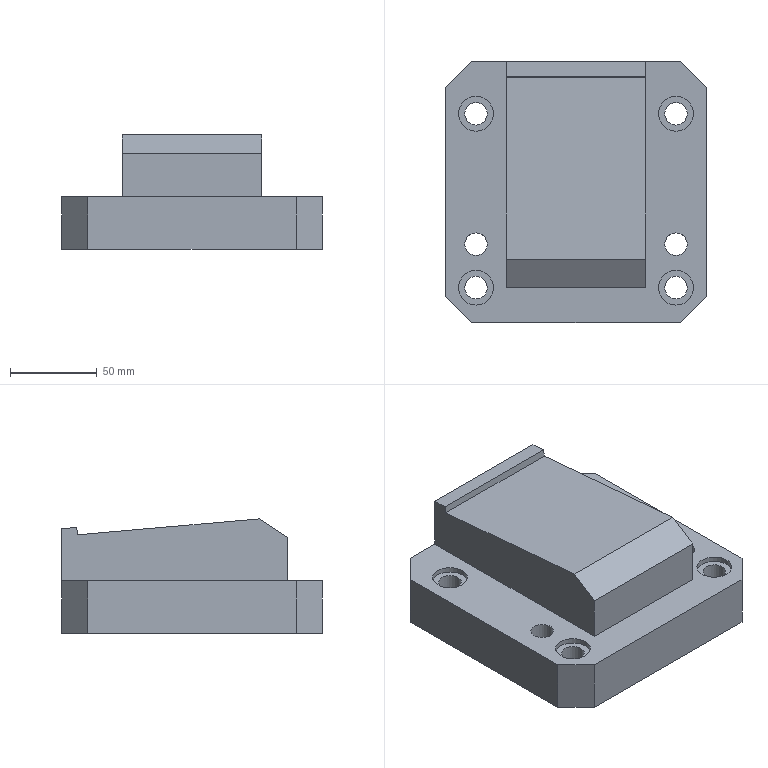Part | NX | features solid 2 | 1 solid | 40 faces | box 150 x 150 x 65.685 mm | volume 939891 mm3 | plane 30 | cylinder 10 | commonest cylinder face diameters 13 x6 20 x4
STEP:
#1=CARTESIAN_POINT('',(197.5,-243.5,-135.));
#2=VERTEX_POINT('',#1);
#3=CARTESIAN_POINT('',(197.5,-250.,-135.));
#4=DIRECTION('',(0.,0.,1.));
#5=DIRECTION('',(0.,1.,0.));
#6=AXIS2_PLACEMENT_3D('',#3,#4,#5);
#7=CIRCLE('',#6,6.5);
#8=EDGE_CURVE('',#2,#2,#7,.T.);
#9=ORIENTED_EDGE('',*,*,#8,.F.);
#10=EDGE_LOOP('',(#9));
#11=FACE_BOUND('',#10,.T.);
#12=CARTESIAN_POINT('',(82.5,-243.5,-135.));
#13=VERTEX_POINT('',#12);
#14=CARTESIAN_POINT('',(82.5,-250.,-135.));
#15=DIRECTION('',(0.,0.,1.));
#16=DIRECTION('',(0.,1.,0.));
#17=AXIS2_PLACEMENT_3D('',#14,#15,#16);
#18=CIRCLE('',#17,6.5);
#19=EDGE_CURVE('',#13,#13,#18,.T.);
#20=ORIENTED_EDGE('',*,*,#19,.F.);
#21=EDGE_LOOP('',(#20));
#22=FACE_BOUND('',#21,.T.);
#23=CARTESIAN_POINT('',(197.5,-265.,-135.));
#24=VERTEX_POINT('',#23);
#25=CARTESIAN_POINT('',(197.5,-275.,-135.));
#26=DIRECTION('',(0.,0.,1.));
#27=DIRECTION('',(0.,1.,0.));
#28=AXIS2_PLACEMENT_3D('',#25,#26,#27);
#29=CIRCLE('',#28,10.);
#30=EDGE_CURVE('',#24,#24,#29,.T.);
#31=ORIENTED_EDGE('',*,*,#30,.F.);
#32=EDGE_LOOP('',(#31));
#33=FACE_BOUND('',#32,.T.);
#34=CARTESIAN_POINT('',(197.5,-165.,-135.));
#35=VERTEX_POINT('',#34);
#36=CARTESIAN_POINT('',(197.5,-175.,-135.));
#37=DIRECTION('',(0.,0.,1.));
#38=DIRECTION('',(0.,1.,0.));
#39=AXIS2_PLACEMENT_3D('',#36,#37,#38);
#40=CIRCLE('',#39,10.);
#41=EDGE_CURVE('',#35,#35,#40,.T.);
#42=ORIENTED_EDGE('',*,*,#41,.F.);
#43=EDGE_LOOP('',(#42));
#44=FACE_BOUND('',#43,.T.);
#45=CARTESIAN_POINT('',(82.5,-165.,-135.));
#46=VERTEX_POINT('',#45);
#47=CARTESIAN_POINT('',(82.5,-175.,-135.));
#48=DIRECTION('',(0.,0.,1.));
#49=DIRECTION('',(0.,1.,0.));
#50=AXIS2_PLACEMENT_3D('',#47,#48,#49);
#51=CIRCLE('',#50,10.);
#52=EDGE_CURVE('',#46,#46,#51,.T.);
#53=ORIENTED_EDGE('',*,*,#52,.F.);
#54=EDGE_LOOP('',(#53));
#55=FACE_BOUND('',#54,.T.);
#56=CARTESIAN_POINT('',(82.5,-265.,-135.));
#57=VERTEX_POINT('',#56);
#58=CARTESIAN_POINT('',(82.5,-275.,-135.));
#59=DIRECTION('',(0.,0.,1.));
#60=DIRECTION('',(0.,1.,0.));
#61=AXIS2_PLACEMENT_3D('',#58,#59,#60);
#62=CIRCLE('',#61,10.);
#63=EDGE_CURVE('',#57,#57,#62,.T.);
#64=ORIENTED_EDGE('',*,*,#63,.F.);
#65=EDGE_LOOP('',(#64));
#66=FACE_BOUND('',#65,.T.);
#67=CARTESIAN_POINT('',(180.,-275.,-135.));
#68=VERTEX_POINT('',#67);
#69=CARTESIAN_POINT('',(100.,-275.,-135.));
#70=VERTEX_POINT('',#69);
#71=CARTESIAN_POINT('',(180.,-275.,-135.));
#72=DIRECTION('',(-1.,0.,0.));
#73=VECTOR('',#72,1000.);
#74=LINE('',#71,#73);
#75=EDGE_CURVE('',#68,#70,#74,.T.);
#76=ORIENTED_EDGE('',*,*,#75,.T.);
#77=CARTESIAN_POINT('',(100.,-145.,-135.));
#78=VERTEX_POINT('',#77);
#79=CARTESIAN_POINT('',(100.,-295.,-135.));
#80=DIRECTION('',(0.,1.,0.));
#81=VECTOR('',#80,1000.);
#82=LINE('',#79,#81);
#83=EDGE_CURVE('',#70,#78,#82,.T.);
#84=ORIENTED_EDGE('',*,*,#83,.T.);
#85=CARTESIAN_POINT('',(80.,-145.,-135.));
#86=VERTEX_POINT('',#85);
#87=CARTESIAN_POINT('',(215.,-145.,-135.));
#88=DIRECTION('',(-1.,0.,0.));
#89=VECTOR('',#88,1000.);
#90=LINE('',#87,#89);
#91=EDGE_CURVE('',#78,#86,#90,.T.);
#92=ORIENTED_EDGE('',*,*,#91,.T.);
#93=CARTESIAN_POINT('',(65.,-160.,-135.));
#94=VERTEX_POINT('',#93);
#95=CARTESIAN_POINT('',(72.5,-152.5,-135.));
#96=DIRECTION('',(0.7071,0.7071,0.));
#97=VECTOR('',#96,1000.);
#98=LINE('',#95,#97);
#99=EDGE_CURVE('',#86,#94,#98,.F.);
#100=ORIENTED_EDGE('',*,*,#99,.T.);
#101=CARTESIAN_POINT('',(65.,-280.,-135.));
#102=VERTEX_POINT('',#101);
#103=CARTESIAN_POINT('',(65.,-295.,-135.));
#104=DIRECTION('',(0.,1.,0.));
#105=VECTOR('',#104,1000.);
#106=LINE('',#103,#105);
#107=EDGE_CURVE('',#102,#94,#106,.T.);
#108=ORIENTED_EDGE('',*,*,#107,.F.);
#109=CARTESIAN_POINT('',(80.,-295.,-135.));
#110=VERTEX_POINT('',#109);
#111=CARTESIAN_POINT('',(147.5,-362.5,-135.));
#112=DIRECTION('',(0.7071,-0.7071,0.));
#113=VECTOR('',#112,1000.);
#114=LINE('',#111,#113);
#115=EDGE_CURVE('',#102,#110,#114,.T.);
#116=ORIENTED_EDGE('',*,*,#115,.T.);
#117=CARTESIAN_POINT('',(200.,-295.,-135.));
#118=VERTEX_POINT('',#117);
#119=CARTESIAN_POINT('',(215.,-295.,-135.));
#120=DIRECTION('',(-1.,0.,0.));
#121=VECTOR('',#120,1000.);
#122=LINE('',#119,#121);
#123=EDGE_CURVE('',#118,#110,#122,.T.);
#124=ORIENTED_EDGE('',*,*,#123,.F.);
#125=CARTESIAN_POINT('',(215.,-280.,-135.));
#126=VERTEX_POINT('',#125);
#127=CARTESIAN_POINT('',(207.5,-287.5,-135.));
#128=DIRECTION('',(-0.7071,-0.7071,0.));
#129=VECTOR('',#128,1000.);
#130=LINE('',#127,#129);
#131=EDGE_CURVE('',#118,#126,#130,.F.);
#132=ORIENTED_EDGE('',*,*,#131,.T.);
#133=CARTESIAN_POINT('',(215.,-160.,-135.));
#134=VERTEX_POINT('',#133);
#135=CARTESIAN_POINT('',(215.,-295.,-135.));
#136=DIRECTION('',(0.,1.,0.));
#137=VECTOR('',#136,1000.);
#138=LINE('',#135,#137);
#139=EDGE_CURVE('',#126,#134,#138,.T.);
#140=ORIENTED_EDGE('',*,*,#139,.T.);
#141=CARTESIAN_POINT('',(200.,-145.,-135.));
#142=VERTEX_POINT('',#141);
#143=CARTESIAN_POINT('',(282.5,-227.5,-135.));
#144=DIRECTION('',(-0.7071,0.7071,0.));
#145=VECTOR('',#144,1000.);
#146=LINE('',#143,#145);
#147=EDGE_CURVE('',#134,#142,#146,.T.);
#148=ORIENTED_EDGE('',*,*,#147,.T.);
#149=CARTESIAN_POINT('',(180.,-145.,-135.));
#150=VERTEX_POINT('',#149);
#151=CARTESIAN_POINT('',(215.,-145.,-135.));
#152=DIRECTION('',(-1.,0.,0.));
#153=VECTOR('',#152,1000.);
#154=LINE('',#151,#153);
#155=EDGE_CURVE('',#142,#150,#154,.T.);
#156=ORIENTED_EDGE('',*,*,#155,.T.);
#157=CARTESIAN_POINT('',(180.,-295.,-135.));
#158=DIRECTION('',(0.,1.,0.));
#159=VECTOR('',#158,1000.);
#160=LINE('',#157,#159);
#161=EDGE_CURVE('',#68,#150,#160,.T.);
#162=ORIENTED_EDGE('',*,*,#161,.F.);
#163=EDGE_LOOP('',(#76,#84,#92,#100,#108,#116,#124,#132,#140,#148,#156,#162));
#164=FACE_BOUND('',#163,.T.);
#165=CARTESIAN_POINT('',(215.,-295.,-135.));
#166=DIRECTION('',(0.,0.,1.));
#167=DIRECTION('',(0.,1.,0.));
#168=AXIS2_PLACEMENT_3D('',#165,#166,#167);
#169=PLANE('',#168);
#170=ADVANCED_FACE('',(#11,#22,#33,#44,#55,#66,#164),#169,.T.);
#171=CARTESIAN_POINT('',(200.,-145.,-165.));
#172=VERTEX_POINT('',#171);
#173=CARTESIAN_POINT('',(80.,-145.,-165.));
#174=VERTEX_POINT('',#173);
#175=CARTESIAN_POINT('',(215.,-145.,-165.));
#176=DIRECTION('',(-1.,0.,0.));
#177=VECTOR('',#176,1000.);
#178=LINE('',#175,#177);
#179=EDGE_CURVE('',#172,#174,#178,.T.);
#180=ORIENTED_EDGE('',*,*,#179,.T.);
#181=CARTESIAN_POINT('',(80.,-145.,-135.));
#182=DIRECTION('',(0.,0.,1.));
#183=VECTOR('',#182,1000.);
#184=LINE('',#181,#183);
#185=EDGE_CURVE('',#174,#86,#184,.T.);
#186=ORIENTED_EDGE('',*,*,#185,.T.);
#187=ORIENTED_EDGE('',*,*,#91,.F.);
#188=CARTESIAN_POINT('',(100.,-145.,-105.));
#189=VERTEX_POINT('',#188);
#190=CARTESIAN_POINT('',(100.,-145.,-135.));
#191=DIRECTION('',(0.,0.,1.));
#192=VECTOR('',#191,1000.);
#193=LINE('',#190,#192);
#194=EDGE_CURVE('',#78,#189,#193,.T.);
#195=ORIENTED_EDGE('',*,*,#194,.T.);
#196=CARTESIAN_POINT('',(180.,-145.,-105.));
#197=VERTEX_POINT('',#196);
#198=CARTESIAN_POINT('',(180.,-145.,-105.));
#199=DIRECTION('',(-1.,0.,0.));
#200=VECTOR('',#199,1000.);
#201=LINE('',#198,#200);
#202=EDGE_CURVE('',#197,#189,#201,.T.);
#203=ORIENTED_EDGE('',*,*,#202,.F.);
#204=CARTESIAN_POINT('',(180.,-145.,-135.));
#205=DIRECTION('',(0.,0.,1.));
#206=VECTOR('',#205,1000.);
#207=LINE('',#204,#206);
#208=EDGE_CURVE('',#150,#197,#207,.T.);
#209=ORIENTED_EDGE('',*,*,#208,.F.);
#210=ORIENTED_EDGE('',*,*,#155,.F.);
#211=CARTESIAN_POINT('',(200.,-145.,-165.));
#212=DIRECTION('',(0.,0.,-1.));
#213=VECTOR('',#212,1000.);
#214=LINE('',#211,#213);
#215=EDGE_CURVE('',#142,#172,#214,.T.);
#216=ORIENTED_EDGE('',*,*,#215,.T.);
#217=EDGE_LOOP('',(#180,#186,#187,#195,#203,#209,#210,#216));
#218=FACE_BOUND('',#217,.T.);
#219=CARTESIAN_POINT('',(215.,-145.,-135.));
#220=DIRECTION('',(0.,1.,0.));
#221=DIRECTION('',(0.,0.,-1.));
#222=AXIS2_PLACEMENT_3D('',#219,#220,#221);
#223=PLANE('',#222);
#224=ADVANCED_FACE('',(#218),#223,.T.);
#225=CARTESIAN_POINT('',(197.5,-181.5,-165.));
#226=VERTEX_POINT('',#225);
#227=CARTESIAN_POINT('',(197.5,-175.,-165.));
#228=DIRECTION('',(0.,0.,-1.));
#229=DIRECTION('',(0.,-1.,0.));
#230=AXIS2_PLACEMENT_3D('',#227,#228,#229);
#231=CIRCLE('',#230,6.5);
#232=EDGE_CURVE('',#226,#226,#231,.T.);
#233=ORIENTED_EDGE('',*,*,#232,.F.);
#234=EDGE_LOOP('',(#233));
#235=FACE_BOUND('',#234,.T.);
#236=CARTESIAN_POINT('',(82.5,-256.5,-165.));
#237=VERTEX_POINT('',#236);
#238=CARTESIAN_POINT('',(82.5,-250.,-165.));
#239=DIRECTION('',(0.,0.,-1.));
#240=DIRECTION('',(0.,-1.,0.));
#241=AXIS2_PLACEMENT_3D('',#238,#239,#240);
#242=CIRCLE('',#241,6.5);
#243=EDGE_CURVE('',#237,#237,#242,.T.);
#244=ORIENTED_EDGE('',*,*,#243,.F.);
#245=EDGE_LOOP('',(#244));
#246=FACE_BOUND('',#245,.T.);
#247=CARTESIAN_POINT('',(82.5,-281.5,-165.));
#248=VERTEX_POINT('',#247);
#249=CARTESIAN_POINT('',(82.5,-275.,-165.));
#250=DIRECTION('',(0.,0.,-1.));
#251=DIRECTION('',(0.,-1.,0.));
#252=AXIS2_PLACEMENT_3D('',#249,#250,#251);
#253=CIRCLE('',#252,6.5);
#254=EDGE_CURVE('',#248,#248,#253,.T.);
#255=ORIENTED_EDGE('',*,*,#254,.F.);
#256=EDGE_LOOP('',(#255));
#257=FACE_BOUND('',#256,.T.);
#258=CARTESIAN_POINT('',(82.5,-181.5,-165.));
#259=VERTEX_POINT('',#258);
#260=CARTESIAN_POINT('',(82.5,-175.,-165.));
#261=DIRECTION('',(0.,0.,-1.));
#262=DIRECTION('',(0.,-1.,0.));
#263=AXIS2_PLACEMENT_3D('',#260,#261,#262);
#264=CIRCLE('',#263,6.5);
#265=EDGE_CURVE('',#259,#259,#264,.T.);
#266=ORIENTED_EDGE('',*,*,#265,.F.);
#267=EDGE_LOOP('',(#266));
#268=FACE_BOUND('',#267,.T.);
#269=CARTESIAN_POINT('',(197.5,-256.5,-165.));
#270=VERTEX_POINT('',#269);
#271=CARTESIAN_POINT('',(197.5,-250.,-165.));
#272=DIRECTION('',(0.,0.,-1.));
#273=DIRECTION('',(0.,-1.,0.));
#274=AXIS2_PLACEMENT_3D('',#271,#272,#273);
#275=CIRCLE('',#274,6.5);
#276=EDGE_CURVE('',#270,#270,#275,.T.);
#277=ORIENTED_EDGE('',*,*,#276,.F.);
#278=EDGE_LOOP('',(#277));
#279=FACE_BOUND('',#278,.T.);
#280=CARTESIAN_POINT('',(197.5,-281.5,-165.));
#281=VERTEX_POINT('',#280);
#282=CARTESIAN_POINT('',(197.5,-275.,-165.));
#283=DIRECTION('',(0.,0.,-1.));
#284=DIRECTION('',(0.,-1.,0.));
#285=AXIS2_PLACEMENT_3D('',#282,#283,#284);
#286=CIRCLE('',#285,6.5);
#287=EDGE_CURVE('',#281,#281,#286,.T.);
#288=ORIENTED_EDGE('',*,*,#287,.F.);
#289=EDGE_LOOP('',(#288));
#290=FACE_BOUND('',#289,.T.);
#291=CARTESIAN_POINT('',(130.,-250.,-165.));
#292=VERTEX_POINT('',#291);
#293=CARTESIAN_POINT('',(125.,-245.,-165.));
#294=VERTEX_POINT('',#293);
#295=CARTESIAN_POINT('',(125.,-245.,-165.));
#296=DIRECTION('',(0.7071,-0.7071,0.));
#297=VECTOR('',#296,1000.);
#298=LINE('',#295,#297);
#299=EDGE_CURVE('',#292,#294,#298,.F.);
#300=ORIENTED_EDGE('',*,*,#299,.F.);
#301=CARTESIAN_POINT('',(150.,-250.,-165.));
#302=VERTEX_POINT('',#301);
#303=CARTESIAN_POINT('',(125.,-250.,-165.));
#304=DIRECTION('',(-1.,0.,0.));
#305=VECTOR('',#304,1000.);
#306=LINE('',#303,#305);
#307=EDGE_CURVE('',#292,#302,#306,.F.);
#308=ORIENTED_EDGE('',*,*,#307,.T.);
#309=CARTESIAN_POINT('',(155.,-245.,-165.));
#310=VERTEX_POINT('',#309);
#311=CARTESIAN_POINT('',(150.,-250.,-165.));
#312=DIRECTION('',(-0.7071,-0.7071,0.));
#313=VECTOR('',#312,1000.);
#314=LINE('',#311,#313);
#315=EDGE_CURVE('',#310,#302,#314,.T.);
#316=ORIENTED_EDGE('',*,*,#315,.F.);
#317=CARTESIAN_POINT('',(155.,-195.,-165.));
#318=VERTEX_POINT('',#317);
#319=CARTESIAN_POINT('',(155.,-160.,-165.));
#320=DIRECTION('',(0.,-1.,0.));
#321=VECTOR('',#320,1000.);
#322=LINE('',#319,#321);
#323=EDGE_CURVE('',#318,#310,#322,.T.);
#324=ORIENTED_EDGE('',*,*,#323,.F.);
#325=CARTESIAN_POINT('',(150.,-190.,-165.));
#326=VERTEX_POINT('',#325);
#327=CARTESIAN_POINT('',(155.,-195.,-165.));
#328=DIRECTION('',(-0.7071,0.7071,0.));
#329=VECTOR('',#328,1000.);
#330=LINE('',#327,#329);
#331=EDGE_CURVE('',#326,#318,#330,.F.);
#332=ORIENTED_EDGE('',*,*,#331,.F.);
#333=CARTESIAN_POINT('',(130.,-190.,-165.));
#334=VERTEX_POINT('',#333);
#335=CARTESIAN_POINT('',(125.,-190.,-165.));
#336=DIRECTION('',(1.,0.,0.));
#337=VECTOR('',#336,1000.);
#338=LINE('',#335,#337);
#339=EDGE_CURVE('',#334,#326,#338,.T.);
#340=ORIENTED_EDGE('',*,*,#339,.F.);
#341=CARTESIAN_POINT('',(125.,-195.,-165.));
#342=VERTEX_POINT('',#341);
#343=CARTESIAN_POINT('',(130.,-190.,-165.));
#344=DIRECTION('',(0.7071,0.7071,0.));
#345=VECTOR('',#344,1000.);
#346=LINE('',#343,#345);
#347=EDGE_CURVE('',#342,#334,#346,.T.);
#348=ORIENTED_EDGE('',*,*,#347,.F.);
#349=CARTESIAN_POINT('',(125.,-160.,-165.));
#350=DIRECTION('',(0.,-1.,0.));
#351=VECTOR('',#350,1000.);
#352=LINE('',#349,#351);
#353=EDGE_CURVE('',#342,#294,#352,.T.);
#354=ORIENTED_EDGE('',*,*,#353,.T.);
#355=EDGE_LOOP('',(#300,#308,#316,#324,#332,#340,#348,#354));
#356=FACE_BOUND('',#355,.T.);
#357=CARTESIAN_POINT('',(200.,-295.,-165.));
#358=VERTEX_POINT('',#357);
#359=CARTESIAN_POINT('',(80.,-295.,-165.));
#360=VERTEX_POINT('',#359);
#361=CARTESIAN_POINT('',(215.,-295.,-165.));
#362=DIRECTION('',(-1.,0.,0.));
#363=VECTOR('',#362,1000.);
#364=LINE('',#361,#363);
#365=EDGE_CURVE('',#358,#360,#364,.T.);
#366=ORIENTED_EDGE('',*,*,#365,.T.);
#367=CARTESIAN_POINT('',(65.,-280.,-165.));
#368=VERTEX_POINT('',#367);
#369=CARTESIAN_POINT('',(72.5,-287.5,-165.));
#370=DIRECTION('',(-0.7071,0.7071,0.));
#371=VECTOR('',#370,1000.);
#372=LINE('',#369,#371);
#373=EDGE_CURVE('',#360,#368,#372,.T.);
#374=ORIENTED_EDGE('',*,*,#373,.T.);
#375=CARTESIAN_POINT('',(65.,-160.,-165.));
#376=VERTEX_POINT('',#375);
#377=CARTESIAN_POINT('',(65.,-145.,-165.));
#378=DIRECTION('',(0.,-1.,0.));
#379=VECTOR('',#378,1000.);
#380=LINE('',#377,#379);
#381=EDGE_CURVE('',#376,#368,#380,.T.);
#382=ORIENTED_EDGE('',*,*,#381,.F.);
#383=CARTESIAN_POINT('',(147.5,-77.5,-165.));
#384=DIRECTION('',(-0.7071,-0.7071,0.));
#385=VECTOR('',#384,1000.);
#386=LINE('',#383,#385);
#387=EDGE_CURVE('',#376,#174,#386,.F.);
#388=ORIENTED_EDGE('',*,*,#387,.T.);
#389=ORIENTED_EDGE('',*,*,#179,.F.);
#390=CARTESIAN_POINT('',(215.,-160.,-165.));
#391=VERTEX_POINT('',#390);
#392=CARTESIAN_POINT('',(207.5,-152.5,-165.));
#393=DIRECTION('',(0.7071,-0.7071,0.));
#394=VECTOR('',#393,1000.);
#395=LINE('',#392,#394);
#396=EDGE_CURVE('',#172,#391,#395,.T.);
#397=ORIENTED_EDGE('',*,*,#396,.T.);
#398=CARTESIAN_POINT('',(215.,-280.,-165.));
#399=VERTEX_POINT('',#398);
#400=CARTESIAN_POINT('',(215.,-145.,-165.));
#401=DIRECTION('',(0.,-1.,0.));
#402=VECTOR('',#401,1000.);
#403=LINE('',#400,#402);
#404=EDGE_CURVE('',#391,#399,#403,.T.);
#405=ORIENTED_EDGE('',*,*,#404,.T.);
#406=CARTESIAN_POINT('',(282.5,-212.5,-165.));
#407=DIRECTION('',(0.7071,0.7071,0.));
#408=VECTOR('',#407,1000.);
#409=LINE('',#406,#408);
#410=EDGE_CURVE('',#399,#358,#409,.F.);
#411=ORIENTED_EDGE('',*,*,#410,.T.);
#412=EDGE_LOOP('',(#366,#374,#382,#388,#389,#397,#405,#411));
#413=FACE_BOUND('',#412,.T.);
#414=CARTESIAN_POINT('',(215.,-145.,-165.));
#415=DIRECTION('',(0.,0.,-1.));
#416=DIRECTION('',(0.,-1.,0.));
#417=AXIS2_PLACEMENT_3D('',#414,#415,#416);
#418=PLANE('',#417);
#419=ADVANCED_FACE('',(#235,#246,#257,#268,#279,#290,#356,#413),#418,.T.);
#420=ORIENTED_EDGE('',*,*,#123,.T.);
#421=CARTESIAN_POINT('',(80.,-295.,-165.));
#422=DIRECTION('',(0.,0.,-1.));
#423=VECTOR('',#422,1000.);
#424=LINE('',#421,#423);
#425=EDGE_CURVE('',#110,#360,#424,.T.);
#426=ORIENTED_EDGE('',*,*,#425,.T.);
#427=ORIENTED_EDGE('',*,*,#365,.F.);
#428=CARTESIAN_POINT('',(200.,-295.,-135.));
#429=DIRECTION('',(0.,0.,1.));
#430=VECTOR('',#429,1000.);
#431=LINE('',#428,#430);
#432=EDGE_CURVE('',#358,#118,#431,.T.);
#433=ORIENTED_EDGE('',*,*,#432,.T.);
#434=EDGE_LOOP('',(#420,#426,#427,#433));
#435=FACE_BOUND('',#434,.T.);
#436=CARTESIAN_POINT('',(215.,-295.,-135.));
#437=DIRECTION('',(0.,1.,0.));
#438=DIRECTION('',(0.,0.,-1.));
#439=AXIS2_PLACEMENT_3D('',#436,#437,#438);
#440=PLANE('',#439);
#441=ADVANCED_FACE('',(#435),#440,.F.);
#442=ORIENTED_EDGE('',*,*,#404,.F.);
#443=CARTESIAN_POINT('',(215.,-160.,-135.));
#444=DIRECTION('',(0.,0.,1.));
#445=VECTOR('',#444,1000.);
#446=LINE('',#443,#445);
#447=EDGE_CURVE('',#391,#134,#446,.T.);
#448=ORIENTED_EDGE('',*,*,#447,.T.);
#449=ORIENTED_EDGE('',*,*,#139,.F.);
#450=CARTESIAN_POINT('',(215.,-280.,-135.));
#451=DIRECTION('',(0.,0.,-1.));
#452=VECTOR('',#451,1000.);
#453=LINE('',#450,#452);
#454=EDGE_CURVE('',#126,#399,#453,.T.);
#455=ORIENTED_EDGE('',*,*,#454,.T.);
#456=EDGE_LOOP('',(#442,#448,#449,#455));
#457=FACE_BOUND('',#456,.T.);
#458=CARTESIAN_POINT('',(215.,-295.,-135.));
#459=DIRECTION('',(-1.,0.,0.));
#460=DIRECTION('',(0.,0.,1.));
#461=AXIS2_PLACEMENT_3D('',#458,#459,#460);
#462=PLANE('',#461);
#463=ADVANCED_FACE('',(#457),#462,.F.);
#464=ORIENTED_EDGE('',*,*,#381,.T.);
#465=CARTESIAN_POINT('',(65.,-280.,-135.));
#466=DIRECTION('',(0.,0.,1.));
#467=VECTOR('',#466,1000.);
#468=LINE('',#465,#467);
#469=EDGE_CURVE('',#368,#102,#468,.T.);
#470=ORIENTED_EDGE('',*,*,#469,.T.);
#471=ORIENTED_EDGE('',*,*,#107,.T.);
#472=CARTESIAN_POINT('',(65.,-160.,-135.));
#473=DIRECTION('',(0.,0.,-1.));
#474=VECTOR('',#473,1000.);
#475=LINE('',#472,#474);
#476=EDGE_CURVE('',#94,#376,#475,.T.);
#477=ORIENTED_EDGE('',*,*,#476,.T.);
#478=EDGE_LOOP('',(#464,#470,#471,#477));
#479=FACE_BOUND('',#478,.T.);
#480=CARTESIAN_POINT('',(65.,-295.,-135.));
#481=DIRECTION('',(-1.,0.,0.));
#482=DIRECTION('',(0.,0.,1.));
#483=AXIS2_PLACEMENT_3D('',#480,#481,#482);
#484=PLANE('',#483);
#485=ADVANCED_FACE('',(#479),#484,.T.);
#486=ORIENTED_EDGE('',*,*,#115,.F.);
#487=ORIENTED_EDGE('',*,*,#469,.F.);
#488=ORIENTED_EDGE('',*,*,#373,.F.);
#489=ORIENTED_EDGE('',*,*,#425,.F.);
#490=EDGE_LOOP('',(#486,#487,#488,#489));
#491=FACE_BOUND('',#490,.T.);
#492=CARTESIAN_POINT('',(80.,-295.,-135.));
#493=DIRECTION('',(-0.7071,-0.7071,0.));
#494=DIRECTION('',(0.7071,-0.7071,0.));
#495=AXIS2_PLACEMENT_3D('',#492,#493,#494);
#496=PLANE('',#495);
#497=ADVANCED_FACE('',(#491),#496,.T.);
#498=ORIENTED_EDGE('',*,*,#99,.F.);
#499=ORIENTED_EDGE('',*,*,#185,.F.);
#500=ORIENTED_EDGE('',*,*,#387,.F.);
#501=ORIENTED_EDGE('',*,*,#476,.F.);
#502=EDGE_LOOP('',(#498,#499,#500,#501));
#503=FACE_BOUND('',#502,.T.);
#504=CARTESIAN_POINT('',(65.,-160.,-135.));
#505=DIRECTION('',(0.7071,-0.7071,0.));
#506=DIRECTION('',(0.7071,0.7071,0.));
#507=AXIS2_PLACEMENT_3D('',#504,#505,#506);
#508=PLANE('',#507);
#509=ADVANCED_FACE('',(#503),#508,.F.);
#510=ORIENTED_EDGE('',*,*,#147,.F.);
#511=ORIENTED_EDGE('',*,*,#447,.F.);
#512=ORIENTED_EDGE('',*,*,#396,.F.);
#513=ORIENTED_EDGE('',*,*,#215,.F.);
#514=EDGE_LOOP('',(#510,#511,#512,#513));
#515=FACE_BOUND('',#514,.T.);
#516=CARTESIAN_POINT('',(200.,-145.,-135.));
#517=DIRECTION('',(0.7071,0.7071,0.));
#518=DIRECTION('',(-0.7071,0.7071,0.));
#519=AXIS2_PLACEMENT_3D('',#516,#517,#518);
#520=PLANE('',#519);
#521=ADVANCED_FACE('',(#515),#520,.T.);
#522=ORIENTED_EDGE('',*,*,#131,.F.);
#523=ORIENTED_EDGE('',*,*,#432,.F.);
#524=ORIENTED_EDGE('',*,*,#410,.F.);
#525=ORIENTED_EDGE('',*,*,#454,.F.);
#526=EDGE_LOOP('',(#522,#523,#524,#525));
#527=FACE_BOUND('',#526,.T.);
#528=CARTESIAN_POINT('',(215.,-280.,-135.));
#529=DIRECTION('',(-0.7071,0.7071,0.));
#530=DIRECTION('',(-0.7071,-0.7071,0.));
#531=AXIS2_PLACEMENT_3D('',#528,#529,#530);
#532=PLANE('',#531);
#533=ADVANCED_FACE('',(#527),#532,.F.);
#534=ORIENTED_EDGE('',*,*,#353,.F.);
#535=CARTESIAN_POINT('',(125.,-195.,-155.));
#536=VERTEX_POINT('',#535);
#537=CARTESIAN_POINT('',(125.,-195.,-165.));
#538=DIRECTION('',(0.,0.,1.));
#539=VECTOR('',#538,1000.);
#540=LINE('',#537,#539);
#541=EDGE_CURVE('',#536,#342,#540,.F.);
#542=ORIENTED_EDGE('',*,*,#541,.F.);
#543=CARTESIAN_POINT('',(125.,-245.,-155.));
#544=VERTEX_POINT('',#543);
#545=CARTESIAN_POINT('',(125.,-160.,-155.));
#546=DIRECTION('',(0.,1.,0.));
#547=VECTOR('',#546,1000.);
#548=LINE('',#545,#547);
#549=EDGE_CURVE('',#536,#544,#548,.F.);
#550=ORIENTED_EDGE('',*,*,#549,.T.);
#551=CARTESIAN_POINT('',(125.,-245.,-165.));
#552=DIRECTION('',(0.,0.,-1.));
#553=VECTOR('',#552,1000.);
#554=LINE('',#551,#553);
#555=EDGE_CURVE('',#294,#544,#554,.F.);
#556=ORIENTED_EDGE('',*,*,#555,.F.);
#557=EDGE_LOOP('',(#534,#542,#550,#556));
#558=FACE_BOUND('',#557,.T.);
#559=CARTESIAN_POINT('',(125.,-160.,-165.));
#560=DIRECTION('',(-1.,0.,0.));
#561=DIRECTION('',(0.,-1.,0.));
#562=AXIS2_PLACEMENT_3D('',#559,#560,#561);
#563=PLANE('',#562);
#564=ADVANCED_FACE('',(#558),#563,.F.);
#565=ORIENTED_EDGE('',*,*,#339,.T.);
#566=CARTESIAN_POINT('',(150.,-190.,-155.));
#567=VERTEX_POINT('',#566);
#568=CARTESIAN_POINT('',(150.,-190.,-165.));
#569=DIRECTION('',(0.,0.,-1.));
#570=VECTOR('',#569,1000.);
#571=LINE('',#568,#570);
#572=EDGE_CURVE('',#567,#326,#571,.T.);
#573=ORIENTED_EDGE('',*,*,#572,.F.);
#574=CARTESIAN_POINT('',(130.,-190.,-155.));
#575=VERTEX_POINT('',#574);
#576=CARTESIAN_POINT('',(125.,-190.,-155.));
#577=DIRECTION('',(1.,0.,0.));
#578=VECTOR('',#577,1000.);
#579=LINE('',#576,#578);
#580=EDGE_CURVE('',#575,#567,#579,.T.);
#581=ORIENTED_EDGE('',*,*,#580,.F.);
#582=CARTESIAN_POINT('',(130.,-190.,-165.));
#583=DIRECTION('',(0.,0.,1.));
#584=VECTOR('',#583,1000.);
#585=LINE('',#582,#584);
#586=EDGE_CURVE('',#334,#575,#585,.T.);
#587=ORIENTED_EDGE('',*,*,#586,.F.);
#588=EDGE_LOOP('',(#565,#573,#581,#587));
#589=FACE_BOUND('',#588,.T.);
#590=CARTESIAN_POINT('',(125.,-190.,-165.));
#591=DIRECTION('',(0.,-1.,0.));
#592=DIRECTION('',(1.,0.,0.));
#593=AXIS2_PLACEMENT_3D('',#590,#591,#592);
#594=PLANE('',#593);
#595=ADVANCED_FACE('',(#589),#594,.T.);
#596=CARTESIAN_POINT('',(155.,-195.,-155.));
#597=VERTEX_POINT('',#596);
#598=CARTESIAN_POINT('',(155.,-245.,-155.));
#599=VERTEX_POINT('',#598);
#600=CARTESIAN_POINT('',(155.,-160.,-155.));
#601=DIRECTION('',(0.,1.,0.));
#602=VECTOR('',#601,1000.);
#603=LINE('',#600,#602);
#604=EDGE_CURVE('',#597,#599,#603,.F.);
#605=ORIENTED_EDGE('',*,*,#604,.F.);
#606=CARTESIAN_POINT('',(155.,-195.,-165.));
#607=DIRECTION('',(0.,0.,1.));
#608=VECTOR('',#607,1000.);
#609=LINE('',#606,#608);
#610=EDGE_CURVE('',#318,#597,#609,.T.);
#611=ORIENTED_EDGE('',*,*,#610,.F.);
#612=ORIENTED_EDGE('',*,*,#323,.T.);
#613=CARTESIAN_POINT('',(155.,-245.,-165.));
#614=DIRECTION('',(0.,0.,-1.));
#615=VECTOR('',#614,1000.);
#616=LINE('',#613,#615);
#617=EDGE_CURVE('',#599,#310,#616,.T.);
#618=ORIENTED_EDGE('',*,*,#617,.F.);
#619=EDGE_LOOP('',(#605,#611,#612,#618));
#620=FACE_BOUND('',#619,.T.);
#621=CARTESIAN_POINT('',(155.,-160.,-165.));
#622=DIRECTION('',(-1.,0.,0.));
#623=DIRECTION('',(0.,-1.,0.));
#624=AXIS2_PLACEMENT_3D('',#621,#622,#623);
#625=PLANE('',#624);
#626=ADVANCED_FACE('',(#620),#625,.T.);
#627=CARTESIAN_POINT('',(130.,-250.,-155.));
#628=VERTEX_POINT('',#627);
#629=CARTESIAN_POINT('',(150.,-250.,-155.));
#630=VERTEX_POINT('',#629);
#631=CARTESIAN_POINT('',(125.,-250.,-155.));
#632=DIRECTION('',(-1.,0.,0.));
#633=VECTOR('',#632,1000.);
#634=LINE('',#631,#633);
#635=EDGE_CURVE('',#628,#630,#634,.F.);
#636=ORIENTED_EDGE('',*,*,#635,.T.);
#637=CARTESIAN_POINT('',(150.,-250.,-165.));
#638=DIRECTION('',(0.,0.,-1.));
#639=VECTOR('',#638,1000.);
#640=LINE('',#637,#639);
#641=EDGE_CURVE('',#302,#630,#640,.F.);
#642=ORIENTED_EDGE('',*,*,#641,.F.);
#643=ORIENTED_EDGE('',*,*,#307,.F.);
#644=CARTESIAN_POINT('',(130.,-250.,-165.));
#645=DIRECTION('',(0.,0.,1.));
#646=VECTOR('',#645,1000.);
#647=LINE('',#644,#646);
#648=EDGE_CURVE('',#628,#292,#647,.F.);
#649=ORIENTED_EDGE('',*,*,#648,.F.);
#650=EDGE_LOOP('',(#636,#642,#643,#649));
#651=FACE_BOUND('',#650,.T.);
#652=CARTESIAN_POINT('',(125.,-250.,-165.));
#653=DIRECTION('',(0.,-1.,0.));
#654=DIRECTION('',(1.,0.,0.));
#655=AXIS2_PLACEMENT_3D('',#652,#653,#654);
#656=PLANE('',#655);
#657=ADVANCED_FACE('',(#651),#656,.F.);
#658=ORIENTED_EDGE('',*,*,#549,.F.);
#659=CARTESIAN_POINT('',(142.5,-177.5,-155.));
#660=DIRECTION('',(-0.7071,-0.7071,0.));
#661=VECTOR('',#660,1000.);
#662=LINE('',#659,#661);
#663=EDGE_CURVE('',#575,#536,#662,.T.);
#664=ORIENTED_EDGE('',*,*,#663,.F.);
#665=ORIENTED_EDGE('',*,*,#580,.T.);
#666=CARTESIAN_POINT('',(122.5,-162.5,-155.));
#667=DIRECTION('',(0.7071,-0.7071,0.));
#668=VECTOR('',#667,1000.);
#669=LINE('',#666,#668);
#670=EDGE_CURVE('',#597,#567,#669,.F.);
#671=ORIENTED_EDGE('',*,*,#670,.F.);
#672=ORIENTED_EDGE('',*,*,#604,.T.);
#673=CARTESIAN_POINT('',(182.5,-217.5,-155.));
#674=DIRECTION('',(0.7071,0.7071,0.));
#675=VECTOR('',#674,1000.);
#676=LINE('',#673,#675);
#677=EDGE_CURVE('',#630,#599,#676,.T.);
#678=ORIENTED_EDGE('',*,*,#677,.F.);
#679=ORIENTED_EDGE('',*,*,#635,.F.);
#680=CARTESIAN_POINT('',(82.5,-202.5,-155.));
#681=DIRECTION('',(-0.7071,0.7071,0.));
#682=VECTOR('',#681,1000.);
#683=LINE('',#680,#682);
#684=EDGE_CURVE('',#544,#628,#683,.F.);
#685=ORIENTED_EDGE('',*,*,#684,.F.);
#686=EDGE_LOOP('',(#658,#664,#665,#671,#672,#678,#679,#685));
#687=FACE_BOUND('',#686,.T.);
#688=CARTESIAN_POINT('',(125.,-160.,-155.));
#689=DIRECTION('',(0.,0.,1.));
#690=DIRECTION('',(0.,1.,0.));
#691=AXIS2_PLACEMENT_3D('',#688,#689,#690);
#692=PLANE('',#691);
#693=ADVANCED_FACE('',(#687),#692,.F.);
#694=ORIENTED_EDGE('',*,*,#299,.T.);
#695=ORIENTED_EDGE('',*,*,#555,.T.);
#696=ORIENTED_EDGE('',*,*,#684,.T.);
#697=ORIENTED_EDGE('',*,*,#648,.T.);
#698=EDGE_LOOP('',(#694,#695,#696,#697));
#699=FACE_BOUND('',#698,.T.);
#700=CARTESIAN_POINT('',(125.,-245.,-165.));
#701=DIRECTION('',(0.7071,0.7071,0.));
#702=DIRECTION('',(-0.7071,0.7071,0.));
#703=AXIS2_PLACEMENT_3D('',#700,#701,#702);
#704=PLANE('',#703);
#705=ADVANCED_FACE('',(#699),#704,.T.);
#706=ORIENTED_EDGE('',*,*,#315,.T.);
#707=ORIENTED_EDGE('',*,*,#641,.T.);
#708=ORIENTED_EDGE('',*,*,#677,.T.);
#709=ORIENTED_EDGE('',*,*,#617,.T.);
#710=EDGE_LOOP('',(#706,#707,#708,#709));
#711=FACE_BOUND('',#710,.T.);
#712=CARTESIAN_POINT('',(150.,-250.,-165.));
#713=DIRECTION('',(0.7071,-0.7071,0.));
#714=DIRECTION('',(0.7071,0.7071,0.));
#715=AXIS2_PLACEMENT_3D('',#712,#713,#714);
#716=PLANE('',#715);
#717=ADVANCED_FACE('',(#711),#716,.F.);
#718=ORIENTED_EDGE('',*,*,#347,.T.);
#719=ORIENTED_EDGE('',*,*,#586,.T.);
#720=ORIENTED_EDGE('',*,*,#663,.T.);
#721=ORIENTED_EDGE('',*,*,#541,.T.);
#722=EDGE_LOOP('',(#718,#719,#720,#721));
#723=FACE_BOUND('',#722,.T.);
#724=CARTESIAN_POINT('',(130.,-190.,-165.));
#725=DIRECTION('',(-0.7071,0.7071,0.));
#726=DIRECTION('',(-0.7071,-0.7071,0.));
#727=AXIS2_PLACEMENT_3D('',#724,#725,#726);
#728=PLANE('',#727);
#729=ADVANCED_FACE('',(#723),#728,.F.);
#730=ORIENTED_EDGE('',*,*,#331,.T.);
#731=ORIENTED_EDGE('',*,*,#610,.T.);
#732=ORIENTED_EDGE('',*,*,#670,.T.);
#733=ORIENTED_EDGE('',*,*,#572,.T.);
#734=EDGE_LOOP('',(#730,#731,#732,#733));
#735=FACE_BOUND('',#734,.T.);
#736=CARTESIAN_POINT('',(155.,-195.,-165.));
#737=DIRECTION('',(-0.7071,-0.7071,0.));
#738=DIRECTION('',(0.7071,-0.7071,0.));
#739=AXIS2_PLACEMENT_3D('',#736,#737,#738);
#740=PLANE('',#739);
#741=ADVANCED_FACE('',(#735),#740,.T.);
#742=CARTESIAN_POINT('',(197.5,-281.5,-138.));
#743=VERTEX_POINT('',#742);
#744=CARTESIAN_POINT('',(197.5,-275.,-138.));
#745=DIRECTION('',(0.,0.,-1.));
#746=DIRECTION('',(0.,-1.,0.));
#747=AXIS2_PLACEMENT_3D('',#744,#745,#746);
#748=CIRCLE('',#747,6.5);
#749=EDGE_CURVE('',#743,#743,#748,.F.);
#750=ORIENTED_EDGE('',*,*,#749,.T.);
#751=EDGE_LOOP('',(#750));
#752=FACE_BOUND('',#751,.T.);
#753=ORIENTED_EDGE('',*,*,#287,.T.);
#754=EDGE_LOOP('',(#753));
#755=FACE_BOUND('',#754,.T.);
#756=CARTESIAN_POINT('',(197.5,-275.,-24.35));
#757=DIRECTION('',(0.,0.,-1.));
#758=DIRECTION('',(0.,-1.,0.));
#759=AXIS2_PLACEMENT_3D('',#756,#757,#758);
#760=CYLINDRICAL_SURFACE('',#759,6.5);
#761=ADVANCED_FACE('',(#752,#755),#760,.F.);
#762=ORIENTED_EDGE('',*,*,#8,.T.);
#763=EDGE_LOOP('',(#762));
#764=FACE_BOUND('',#763,.T.);
#765=ORIENTED_EDGE('',*,*,#276,.T.);
#766=EDGE_LOOP('',(#765));
#767=FACE_BOUND('',#766,.T.);
#768=CARTESIAN_POINT('',(197.5,-250.,-24.35));
#769=DIRECTION('',(0.,0.,-1.));
#770=DIRECTION('',(0.,-1.,0.));
#771=AXIS2_PLACEMENT_3D('',#768,#769,#770);
#772=CYLINDRICAL_SURFACE('',#771,6.5);
#773=ADVANCED_FACE('',(#764,#767),#772,.F.);
#774=CARTESIAN_POINT('',(82.5,-181.5,-138.));
#775=VERTEX_POINT('',#774);
#776=CARTESIAN_POINT('',(82.5,-175.,-138.));
#777=DIRECTION('',(0.,0.,-1.));
#778=DIRECTION('',(0.,-1.,0.));
#779=AXIS2_PLACEMENT_3D('',#776,#777,#778);
#780=CIRCLE('',#779,6.5);
#781=EDGE_CURVE('',#775,#775,#780,.F.);
#782=ORIENTED_EDGE('',*,*,#781,.T.);
#783=EDGE_LOOP('',(#782));
#784=FACE_BOUND('',#783,.T.);
#785=ORIENTED_EDGE('',*,*,#265,.T.);
#786=EDGE_LOOP('',(#785));
#787=FACE_BOUND('',#786,.T.);
#788=CARTESIAN_POINT('',(82.5,-175.,-24.35));
#789=DIRECTION('',(0.,0.,-1.));
#790=DIRECTION('',(0.,-1.,0.));
#791=AXIS2_PLACEMENT_3D('',#788,#789,#790);
#792=CYLINDRICAL_SURFACE('',#791,6.5);
#793=ADVANCED_FACE('',(#784,#787),#792,.F.);
#794=CARTESIAN_POINT('',(82.5,-281.5,-138.));
#795=VERTEX_POINT('',#794);
#796=CARTESIAN_POINT('',(82.5,-275.,-138.));
#797=DIRECTION('',(0.,0.,-1.));
#798=DIRECTION('',(0.,-1.,0.));
#799=AXIS2_PLACEMENT_3D('',#796,#797,#798);
#800=CIRCLE('',#799,6.5);
#801=EDGE_CURVE('',#795,#795,#800,.F.);
#802=ORIENTED_EDGE('',*,*,#801,.T.);
#803=EDGE_LOOP('',(#802));
#804=FACE_BOUND('',#803,.T.);
#805=ORIENTED_EDGE('',*,*,#254,.T.);
#806=EDGE_LOOP('',(#805));
#807=FACE_BOUND('',#806,.T.);
#808=CARTESIAN_POINT('',(82.5,-275.,-24.35));
#809=DIRECTION('',(0.,0.,-1.));
#810=DIRECTION('',(0.,-1.,0.));
#811=AXIS2_PLACEMENT_3D('',#808,#809,#810);
#812=CYLINDRICAL_SURFACE('',#811,6.5);
#813=ADVANCED_FACE('',(#804,#807),#812,.F.);
#814=ORIENTED_EDGE('',*,*,#19,.T.);
#815=EDGE_LOOP('',(#814));
#816=FACE_BOUND('',#815,.T.);
#817=ORIENTED_EDGE('',*,*,#243,.T.);
#818=EDGE_LOOP('',(#817));
#819=FACE_BOUND('',#818,.T.);
#820=CARTESIAN_POINT('',(82.5,-250.,-24.35));
#821=DIRECTION('',(0.,0.,-1.));
#822=DIRECTION('',(0.,-1.,0.));
#823=AXIS2_PLACEMENT_3D('',#820,#821,#822);
#824=CYLINDRICAL_SURFACE('',#823,6.5);
#825=ADVANCED_FACE('',(#816,#819),#824,.F.);
#826=CARTESIAN_POINT('',(197.5,-181.5,-138.));
#827=VERTEX_POINT('',#826);
#828=CARTESIAN_POINT('',(197.5,-175.,-138.));
#829=DIRECTION('',(0.,0.,-1.));
#830=DIRECTION('',(0.,-1.,0.));
#831=AXIS2_PLACEMENT_3D('',#828,#829,#830);
#832=CIRCLE('',#831,6.5);
#833=EDGE_CURVE('',#827,#827,#832,.F.);
#834=ORIENTED_EDGE('',*,*,#833,.T.);
#835=EDGE_LOOP('',(#834));
#836=FACE_BOUND('',#835,.T.);
#837=ORIENTED_EDGE('',*,*,#232,.T.);
#838=EDGE_LOOP('',(#837));
#839=FACE_BOUND('',#838,.T.);
#840=CARTESIAN_POINT('',(197.5,-175.,-24.35));
#841=DIRECTION('',(0.,0.,-1.));
#842=DIRECTION('',(0.,-1.,0.));
#843=AXIS2_PLACEMENT_3D('',#840,#841,#842);
#844=CYLINDRICAL_SURFACE('',#843,6.5);
#845=ADVANCED_FACE('',(#836,#839),#844,.F.);
#846=CARTESIAN_POINT('',(197.5,-265.,-138.));
#847=VERTEX_POINT('',#846);
#848=CARTESIAN_POINT('',(197.5,-275.,-138.));
#849=DIRECTION('',(0.,0.,-1.));
#850=DIRECTION('',(0.,1.,0.));
#851=AXIS2_PLACEMENT_3D('',#848,#849,#850);
#852=CIRCLE('',#851,10.);
#853=EDGE_CURVE('',#847,#847,#852,.T.);
#854=ORIENTED_EDGE('',*,*,#853,.F.);
#855=EDGE_LOOP('',(#854));
#856=FACE_BOUND('',#855,.T.);
#857=ORIENTED_EDGE('',*,*,#749,.F.);
#858=EDGE_LOOP('',(#857));
#859=FACE_BOUND('',#858,.T.);
#860=CARTESIAN_POINT('',(197.5,-275.,-138.));
#861=DIRECTION('',(0.,0.,-1.));
#862=DIRECTION('',(0.,-1.,0.));
#863=AXIS2_PLACEMENT_3D('',#860,#861,#862);
#864=PLANE('',#863);
#865=ADVANCED_FACE('',(#856,#859),#864,.F.);
#866=ORIENTED_EDGE('',*,*,#30,.T.);
#867=EDGE_LOOP('',(#866));
#868=FACE_BOUND('',#867,.T.);
#869=ORIENTED_EDGE('',*,*,#853,.T.);
#870=EDGE_LOOP('',(#869));
#871=FACE_BOUND('',#870,.T.);
#872=CARTESIAN_POINT('',(197.5,-275.,-24.35));
#873=DIRECTION('',(0.,0.,-1.));
#874=DIRECTION('',(0.,-1.,0.));
#875=AXIS2_PLACEMENT_3D('',#872,#873,#874);
#876=CYLINDRICAL_SURFACE('',#875,10.);
#877=ADVANCED_FACE('',(#868,#871),#876,.F.);
#878=CARTESIAN_POINT('',(197.5,-165.,-138.));
#879=VERTEX_POINT('',#878);
#880=CARTESIAN_POINT('',(197.5,-175.,-138.));
#881=DIRECTION('',(0.,0.,-1.));
#882=DIRECTION('',(0.,1.,0.));
#883=AXIS2_PLACEMENT_3D('',#880,#881,#882);
#884=CIRCLE('',#883,10.);
#885=EDGE_CURVE('',#879,#879,#884,.T.);
#886=ORIENTED_EDGE('',*,*,#885,.F.);
#887=EDGE_LOOP('',(#886));
#888=FACE_BOUND('',#887,.T.);
#889=ORIENTED_EDGE('',*,*,#833,.F.);
#890=EDGE_LOOP('',(#889));
#891=FACE_BOUND('',#890,.T.);
#892=CARTESIAN_POINT('',(197.5,-175.,-138.));
#893=DIRECTION('',(0.,0.,-1.));
#894=DIRECTION('',(0.,-1.,0.));
#895=AXIS2_PLACEMENT_3D('',#892,#893,#894);
#896=PLANE('',#895);
#897=ADVANCED_FACE('',(#888,#891),#896,.F.);
#898=ORIENTED_EDGE('',*,*,#41,.T.);
#899=EDGE_LOOP('',(#898));
#900=FACE_BOUND('',#899,.T.);
#901=ORIENTED_EDGE('',*,*,#885,.T.);
#902=EDGE_LOOP('',(#901));
#903=FACE_BOUND('',#902,.T.);
#904=CARTESIAN_POINT('',(197.5,-175.,-24.35));
#905=DIRECTION('',(0.,0.,-1.));
#906=DIRECTION('',(0.,-1.,0.));
#907=AXIS2_PLACEMENT_3D('',#904,#905,#906);
#908=CYLINDRICAL_SURFACE('',#907,10.);
#909=ADVANCED_FACE('',(#900,#903),#908,.F.);
#910=CARTESIAN_POINT('',(82.5,-165.,-138.));
#911=VERTEX_POINT('',#910);
#912=CARTESIAN_POINT('',(82.5,-175.,-138.));
#913=DIRECTION('',(0.,0.,-1.));
#914=DIRECTION('',(0.,1.,0.));
#915=AXIS2_PLACEMENT_3D('',#912,#913,#914);
#916=CIRCLE('',#915,10.);
#917=EDGE_CURVE('',#911,#911,#916,.T.);
#918=ORIENTED_EDGE('',*,*,#917,.F.);
#919=EDGE_LOOP('',(#918));
#920=FACE_BOUND('',#919,.T.);
#921=ORIENTED_EDGE('',*,*,#781,.F.);
#922=EDGE_LOOP('',(#921));
#923=FACE_BOUND('',#922,.T.);
#924=CARTESIAN_POINT('',(82.5,-175.,-138.));
#925=DIRECTION('',(0.,0.,-1.));
#926=DIRECTION('',(0.,-1.,0.));
#927=AXIS2_PLACEMENT_3D('',#924,#925,#926);
#928=PLANE('',#927);
#929=ADVANCED_FACE('',(#920,#923),#928,.F.);
#930=ORIENTED_EDGE('',*,*,#52,.T.);
#931=EDGE_LOOP('',(#930));
#932=FACE_BOUND('',#931,.T.);
#933=ORIENTED_EDGE('',*,*,#917,.T.);
#934=EDGE_LOOP('',(#933));
#935=FACE_BOUND('',#934,.T.);
#936=CARTESIAN_POINT('',(82.5,-175.,-24.35));
#937=DIRECTION('',(0.,0.,-1.));
#938=DIRECTION('',(0.,-1.,0.));
#939=AXIS2_PLACEMENT_3D('',#936,#937,#938);
#940=CYLINDRICAL_SURFACE('',#939,10.);
#941=ADVANCED_FACE('',(#932,#935),#940,.F.);
#942=CARTESIAN_POINT('',(82.5,-265.,-138.));
#943=VERTEX_POINT('',#942);
#944=CARTESIAN_POINT('',(82.5,-275.,-138.));
#945=DIRECTION('',(0.,0.,-1.));
#946=DIRECTION('',(0.,1.,0.));
#947=AXIS2_PLACEMENT_3D('',#944,#945,#946);
#948=CIRCLE('',#947,10.);
#949=EDGE_CURVE('',#943,#943,#948,.T.);
#950=ORIENTED_EDGE('',*,*,#949,.F.);
#951=EDGE_LOOP('',(#950));
#952=FACE_BOUND('',#951,.T.);
#953=ORIENTED_EDGE('',*,*,#801,.F.);
#954=EDGE_LOOP('',(#953));
#955=FACE_BOUND('',#954,.T.);
#956=CARTESIAN_POINT('',(82.5,-275.,-138.));
#957=DIRECTION('',(0.,0.,-1.));
#958=DIRECTION('',(0.,-1.,0.));
#959=AXIS2_PLACEMENT_3D('',#956,#957,#958);
#960=PLANE('',#959);
#961=ADVANCED_FACE('',(#952,#955),#960,.F.);
#962=ORIENTED_EDGE('',*,*,#63,.T.);
#963=EDGE_LOOP('',(#962));
#964=FACE_BOUND('',#963,.T.);
#965=ORIENTED_EDGE('',*,*,#949,.T.);
#966=EDGE_LOOP('',(#965));
#967=FACE_BOUND('',#966,.T.);
#968=CARTESIAN_POINT('',(82.5,-275.,-24.35));
#969=DIRECTION('',(0.,0.,-1.));
#970=DIRECTION('',(0.,-1.,0.));
#971=AXIS2_PLACEMENT_3D('',#968,#969,#970);
#972=CYLINDRICAL_SURFACE('',#971,10.);
#973=ADVANCED_FACE('',(#964,#967),#972,.F.);
#974=CARTESIAN_POINT('',(100.,-275.,-110.));
#975=VERTEX_POINT('',#974);
#976=CARTESIAN_POINT('',(100.,-275.,-110.));
#977=DIRECTION('',(0.,0.,-1.));
#978=VECTOR('',#977,1000.);
#979=LINE('',#976,#978);
#980=EDGE_CURVE('',#975,#70,#979,.T.);
#981=ORIENTED_EDGE('',*,*,#980,.T.);
#982=ORIENTED_EDGE('',*,*,#75,.F.);
#983=CARTESIAN_POINT('',(180.,-275.,-110.));
#984=VERTEX_POINT('',#983);
#985=CARTESIAN_POINT('',(180.,-275.,-110.));
#986=DIRECTION('',(0.,0.,-1.));
#987=VECTOR('',#986,1000.);
#988=LINE('',#985,#987);
#989=EDGE_CURVE('',#984,#68,#988,.T.);
#990=ORIENTED_EDGE('',*,*,#989,.F.);
#991=CARTESIAN_POINT('',(180.,-275.,-110.));
#992=DIRECTION('',(-1.,0.,0.));
#993=VECTOR('',#992,1000.);
#994=LINE('',#991,#993);
#995=EDGE_CURVE('',#984,#975,#994,.T.);
#996=ORIENTED_EDGE('',*,*,#995,.T.);
#997=EDGE_LOOP('',(#981,#982,#990,#996));
#998=FACE_BOUND('',#997,.T.);
#999=CARTESIAN_POINT('',(180.,-275.,-110.));
#1000=DIRECTION('',(0.,1.,0.));
#1001=DIRECTION('',(0.,0.,-1.));
#1002=AXIS2_PLACEMENT_3D('',#999,#1000,#1001);
#1003=PLANE('',#1002);
#1004=ADVANCED_FACE('',(#998),#1003,.F.);
#1005=CARTESIAN_POINT('',(100.,-258.715,-99.315));
#1006=VERTEX_POINT('',#1005);
#1007=CARTESIAN_POINT('',(100.,-275.,-110.));
#1008=DIRECTION('',(0.,0.8361,0.5486));
#1009=VECTOR('',#1008,1000.);
#1010=LINE('',#1007,#1009);
#1011=EDGE_CURVE('',#975,#1006,#1010,.T.);
#1012=ORIENTED_EDGE('',*,*,#1011,.F.);
#1013=ORIENTED_EDGE('',*,*,#995,.F.);
#1014=CARTESIAN_POINT('',(180.,-258.715,-99.315));
#1015=VERTEX_POINT('',#1014);
#1016=CARTESIAN_POINT('',(180.,-275.,-110.));
#1017=DIRECTION('',(0.,0.8361,0.5486));
#1018=VECTOR('',#1017,1000.);
#1019=LINE('',#1016,#1018);
#1020=EDGE_CURVE('',#984,#1015,#1019,.T.);
#1021=ORIENTED_EDGE('',*,*,#1020,.T.);
#1022=CARTESIAN_POINT('',(180.,-258.715,-99.315));
#1023=DIRECTION('',(-1.,0.,0.));
#1024=VECTOR('',#1023,1000.);
#1025=LINE('',#1022,#1024);
#1026=EDGE_CURVE('',#1015,#1006,#1025,.T.);
#1027=ORIENTED_EDGE('',*,*,#1026,.T.);
#1028=EDGE_LOOP('',(#1012,#1013,#1021,#1027));
#1029=FACE_BOUND('',#1028,.T.);
#1030=CARTESIAN_POINT('',(180.,-275.,-110.));
#1031=DIRECTION('',(0.,-0.5486,0.8361));
#1032=DIRECTION('',(0.,0.8361,0.5486));
#1033=AXIS2_PLACEMENT_3D('',#1030,#1031,#1032);
#1034=PLANE('',#1033);
#1035=ADVANCED_FACE('',(#1029),#1034,.T.);
#1036=CARTESIAN_POINT('',(100.,-154.115,-108.466));
#1037=VERTEX_POINT('',#1036);
#1038=CARTESIAN_POINT('',(100.,-258.715,-99.315));
#1039=DIRECTION('',(0.,0.9962,-0.08716));
#1040=VECTOR('',#1039,1000.);
#1041=LINE('',#1038,#1040);
#1042=EDGE_CURVE('',#1006,#1037,#1041,.T.);
#1043=ORIENTED_EDGE('',*,*,#1042,.F.);
#1044=ORIENTED_EDGE('',*,*,#1026,.F.);
#1045=CARTESIAN_POINT('',(180.,-154.115,-108.466));
#1046=VERTEX_POINT('',#1045);
#1047=CARTESIAN_POINT('',(180.,-258.715,-99.315));
#1048=DIRECTION('',(0.,0.9962,-0.08716));
#1049=VECTOR('',#1048,1000.);
#1050=LINE('',#1047,#1049);
#1051=EDGE_CURVE('',#1015,#1046,#1050,.T.);
#1052=ORIENTED_EDGE('',*,*,#1051,.T.);
#1053=CARTESIAN_POINT('',(180.,-154.115,-108.466));
#1054=DIRECTION('',(-1.,0.,0.));
#1055=VECTOR('',#1054,1000.);
#1056=LINE('',#1053,#1055);
#1057=EDGE_CURVE('',#1046,#1037,#1056,.T.);
#1058=ORIENTED_EDGE('',*,*,#1057,.T.);
#1059=EDGE_LOOP('',(#1043,#1044,#1052,#1058));
#1060=FACE_BOUND('',#1059,.T.);
#1061=CARTESIAN_POINT('',(180.,-258.715,-99.315));
#1062=DIRECTION('',(0.,0.08716,0.9962));
#1063=DIRECTION('',(0.,0.9962,-0.08716));
#1064=AXIS2_PLACEMENT_3D('',#1061,#1062,#1063);
#1065=PLANE('',#1064);
#1066=ADVANCED_FACE('',(#1060),#1065,.T.);
#1067=CARTESIAN_POINT('',(100.,-153.745,-104.235));
#1068=VERTEX_POINT('',#1067);
#1069=CARTESIAN_POINT('',(100.,-151.5,-78.58));
#1070=DIRECTION('',(0.,-0.08716,-0.9962));
#1071=VECTOR('',#1070,1000.);
#1072=LINE('',#1069,#1071);
#1073=EDGE_CURVE('',#1068,#1037,#1072,.T.);
#1074=ORIENTED_EDGE('',*,*,#1073,.T.);
#1075=ORIENTED_EDGE('',*,*,#1057,.F.);
#1076=CARTESIAN_POINT('',(180.,-153.745,-104.235));
#1077=VERTEX_POINT('',#1076);
#1078=CARTESIAN_POINT('',(180.,-151.5,-78.58));
#1079=DIRECTION('',(0.,-0.08716,-0.9962));
#1080=VECTOR('',#1079,1000.);
#1081=LINE('',#1078,#1080);
#1082=EDGE_CURVE('',#1077,#1046,#1081,.T.);
#1083=ORIENTED_EDGE('',*,*,#1082,.F.);
#1084=CARTESIAN_POINT('',(180.,-153.745,-104.235));
#1085=DIRECTION('',(-1.,0.,0.));
#1086=VECTOR('',#1085,1000.);
#1087=LINE('',#1084,#1086);
#1088=EDGE_CURVE('',#1077,#1068,#1087,.T.);
#1089=ORIENTED_EDGE('',*,*,#1088,.T.);
#1090=EDGE_LOOP('',(#1074,#1075,#1083,#1089));
#1091=FACE_BOUND('',#1090,.T.);
#1092=CARTESIAN_POINT('',(180.,-151.5,-78.58));
#1093=DIRECTION('',(0.,0.9962,-0.08716));
#1094=DIRECTION('',(0.,-0.08716,-0.9962));
#1095=AXIS2_PLACEMENT_3D('',#1092,#1093,#1094);
#1096=PLANE('',#1095);
#1097=ADVANCED_FACE('',(#1091),#1096,.F.);
#1098=CARTESIAN_POINT('',(100.,-145.,-105.));
#1099=DIRECTION('',(0.,-0.9962,0.08716));
#1100=VECTOR('',#1099,1000.);
#1101=LINE('',#1098,#1100);
#1102=EDGE_CURVE('',#189,#1068,#1101,.T.);
#1103=ORIENTED_EDGE('',*,*,#1102,.T.);
#1104=ORIENTED_EDGE('',*,*,#1088,.F.);
#1105=CARTESIAN_POINT('',(180.,-145.,-105.));
#1106=DIRECTION('',(0.,-0.9962,0.08716));
#1107=VECTOR('',#1106,1000.);
#1108=LINE('',#1105,#1107);
#1109=EDGE_CURVE('',#197,#1077,#1108,.T.);
#1110=ORIENTED_EDGE('',*,*,#1109,.F.);
#1111=ORIENTED_EDGE('',*,*,#202,.T.);
#1112=EDGE_LOOP('',(#1103,#1104,#1110,#1111));
#1113=FACE_BOUND('',#1112,.T.);
#1114=CARTESIAN_POINT('',(180.,-145.,-105.));
#1115=DIRECTION('',(0.,-0.08716,-0.9962));
#1116=DIRECTION('',(0.,-0.9962,0.08716));
#1117=AXIS2_PLACEMENT_3D('',#1114,#1115,#1116);
#1118=PLANE('',#1117);
#1119=ADVANCED_FACE('',(#1113),#1118,.F.);
#1120=ORIENTED_EDGE('',*,*,#989,.T.);
#1121=ORIENTED_EDGE('',*,*,#161,.T.);
#1122=ORIENTED_EDGE('',*,*,#208,.T.);
#1123=ORIENTED_EDGE('',*,*,#1109,.T.);
#1124=ORIENTED_EDGE('',*,*,#1082,.T.);
#1125=ORIENTED_EDGE('',*,*,#1051,.F.);
#1126=ORIENTED_EDGE('',*,*,#1020,.F.);
#1127=EDGE_LOOP('',(#1120,#1121,#1122,#1123,#1124,#1125,#1126));
#1128=FACE_BOUND('',#1127,.T.);
#1129=CARTESIAN_POINT('',(180.,-202.208,-112.027));
#1130=DIRECTION('',(-1.,0.,0.));
#1131=DIRECTION('',(0.,0.,1.));
#1132=AXIS2_PLACEMENT_3D('',#1129,#1130,#1131);
#1133=PLANE('',#1132);
#1134=ADVANCED_FACE('',(#1128),#1133,.F.);
#1135=ORIENTED_EDGE('',*,*,#980,.F.);
#1136=ORIENTED_EDGE('',*,*,#1011,.T.);
#1137=ORIENTED_EDGE('',*,*,#1042,.T.);
#1138=ORIENTED_EDGE('',*,*,#1073,.F.);
#1139=ORIENTED_EDGE('',*,*,#1102,.F.);
#1140=ORIENTED_EDGE('',*,*,#194,.F.);
#1141=ORIENTED_EDGE('',*,*,#83,.F.);
#1142=EDGE_LOOP('',(#1135,#1136,#1137,#1138,#1139,#1140,#1141));
#1143=FACE_BOUND('',#1142,.T.);
#1144=CARTESIAN_POINT('',(100.,-202.208,-112.027));
#1145=DIRECTION('',(-1.,0.,0.));
#1146=DIRECTION('',(0.,0.,1.));
#1147=AXIS2_PLACEMENT_3D('',#1144,#1145,#1146);
#1148=PLANE('',#1147);
#1149=ADVANCED_FACE('',(#1143),#1148,.T.);
#1150=CLOSED_SHELL('',(#170,#224,#419,#441,#463,#485,#497,#509,#521,#533,#564,#595,#626,#657,#693,#705,#717,#729,#741,#761,#773,#793,#813,#825,#845,#865,#877,#897,#909,#929,#941,#961,#973,#1004,#1035,#1066,#1097,#1119,#1134,#1149));
#1151=MANIFOLD_SOLID_BREP('',#1150);
#1152=(LENGTH_UNIT()NAMED_UNIT(*)SI_UNIT(.MILLI.,.METRE.));
#1153=UNCERTAINTY_MEASURE_WITH_UNIT(LENGTH_MEASURE(0.00001),#1152,'','');
#1154=(NAMED_UNIT(*)PLANE_ANGLE_UNIT()SI_UNIT($,.RADIAN.));
#1155=(NAMED_UNIT(*)SI_UNIT($,.STERADIAN.)SOLID_ANGLE_UNIT());
#1156=(GEOMETRIC_REPRESENTATION_CONTEXT(3)GLOBAL_UNCERTAINTY_ASSIGNED_CONTEXT((#1153))GLOBAL_UNIT_ASSIGNED_CONTEXT((#1152,#1154,#1155))REPRESENTATION_CONTEXT('',''));
#1157=ADVANCED_BREP_SHAPE_REPRESENTATION('',(#1151),#1156);